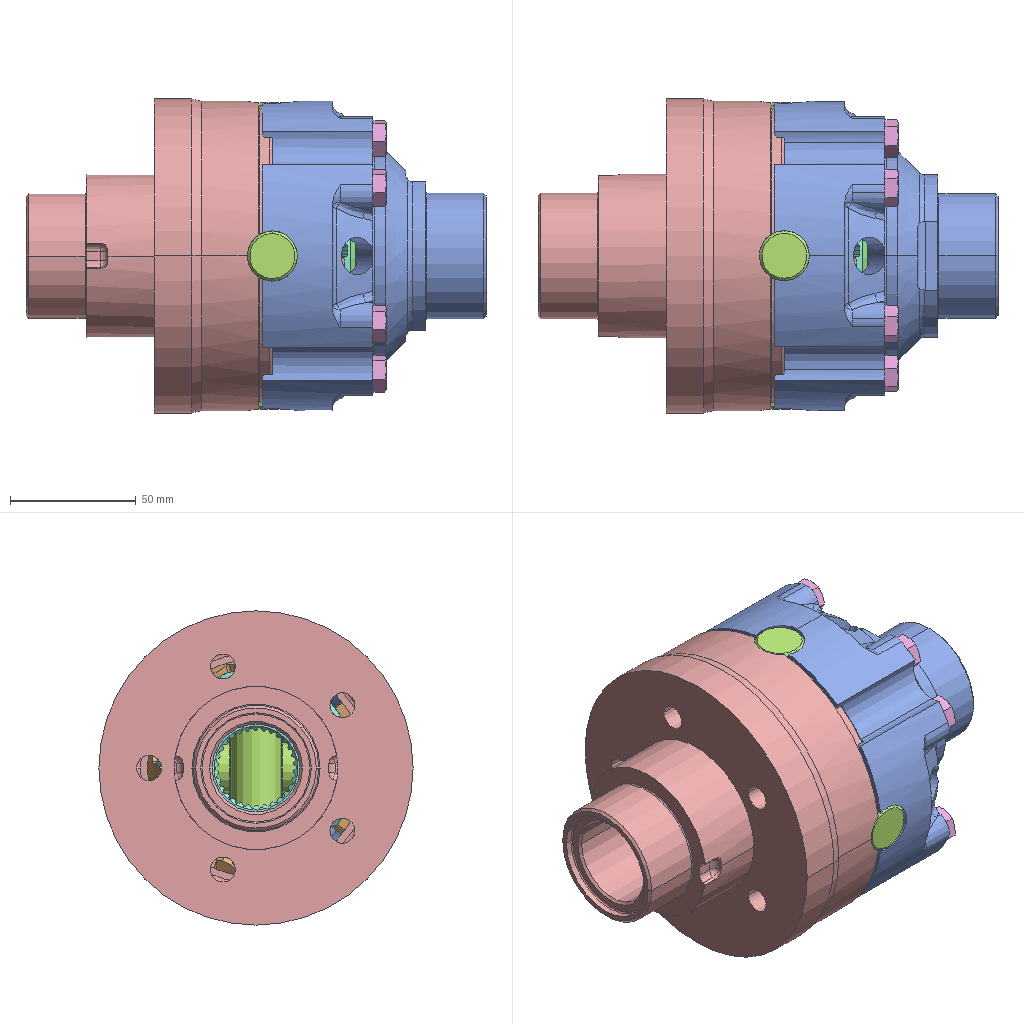Assembly | SolidWorks | 8 different items | 17 placed | box 183 x 125 x 125 mm
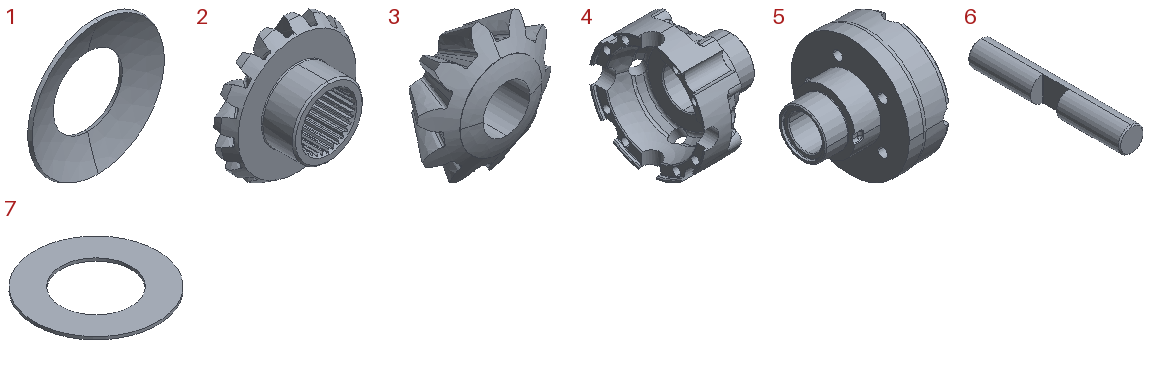Parts list (item | name | quantity | size | volume | features):
1 | - | x4 | 40 x 4.084 x 40 mm | 947.141 mm3 | features Revolution 1
2 | - | x2 | 78.97 x 37 x 78.97 mm | 57789 mm3 | features BaseBody 1
3 | - | x4 | 57.348 x 25.263 x 57.563 mm | 22124 mm3 | features BaseBody 1
4 | - | x1 | 89 x 123 x 123 mm | 266292 mm3 | features Cut 5, Fillet 3, CirPattern 2, Chamfer 1, RevCut 1, Revolution 1
5 | - | x1 | 98 x 125 x 125 mm | 341274 mm3 | features Fillet 5, Cut 4, Draft 3, ICE 3, CirPattern 2, Chamfer 1, HoleWzd 1, Revolution 1
6 | - | x2 | 20 x 122 x 20 mm | 34970 mm3 | features Chamfer 1, Cut 1, Extrusion 1
7 | - | x2 | 74 x 74 x 1.71 mm | 4985 mm3 | features Extrusion 1
8 | hex bolt gradeb_din | x1 | - | - | -
Mates (type | each side: item.copy, entity, surface, feature):
Concentric | 5.1 face cylinder CirPattern2 | 6.1 face cylinder Boss-Extrude1
Coincident | 6.2 face plane Cut-Extrude1 | 6.1 face plane Cut-Extrude1
Symmetric | 6.1 face plane Cut-Extrude1 | 6.1 face plane Cut-Extrude1 | assembly plane
Concentric | 5.1 face cylinder Revolve1 | 2.1 face cylinder Imported1
DistanceDim | 2.1 face plane Imported1 | 5.1 face plane Revolve1
Concentric | 4.1 face cylinder Revolve1 | 2.2 face cylinder Imported1
DistanceDim | 2.2 face plane Imported1 | 4.1 face plane Revolve1
Concentric | 6.2 face cylinder Boss-Extrude1 | 3.1 face cylinder Imported1
Concentric | 6.2 face cylinder Boss-Extrude1 | 1.1 edge
Concentric | 5.1 face sphere Revolve1 | 1.1 face sphere Revolve1
Tangent | 3.1 face surface:4010 Imported1 | 1.1 face sphere Revolve1
Concentric | 2.1 face cylinder Imported1 | 7.1 face cylinder Boss-Extrude1
Coincident | 2.1 face plane Imported1 | 7.1 face plane Boss-Extrude1
Concentric | 2.2 face cylinder Imported1 | 7.2 face cylinder Boss-Extrude1
Coincident | 2.2 face plane Imported1 | 7.2 face plane Boss-Extrude1